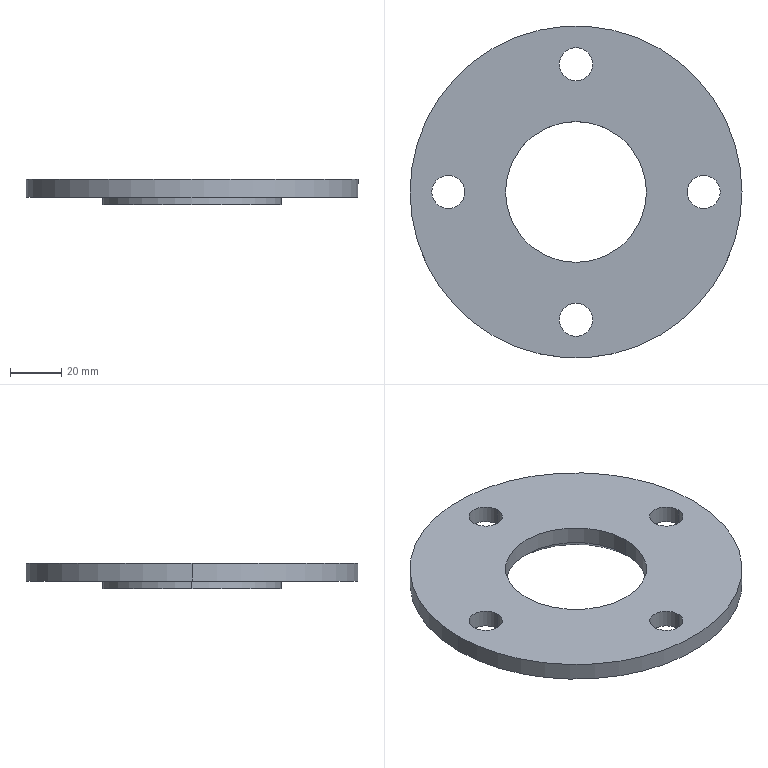Part | SolidWorks | features BaseBody 1 | 1 solid | 19 faces | box 130 x 130 x 10 mm | volume 76001 mm3 | cylinder 14 | plane 3 | cone 2 | commonest cylinder face diameters 13 x8 55.2 x2 70 x2 130 x2
STEP:
#1=CARTESIAN_POINT('',(27.6,0.,-7.));
#2=VERTEX_POINT('',#1);
#3=CARTESIAN_POINT('',(30.6,0.,-10.));
#4=VERTEX_POINT('',#3);
#5=CARTESIAN_POINT('',(30.6,0.,-10.));
#6=DIRECTION('',(0.7071,0.,-0.7071));
#7=VECTOR('',#6,1000.);
#8=LINE('',#5,#7);
#9=EDGE_CURVE('',#2,#4,#8,.T.);
#10=ORIENTED_EDGE('',*,*,#9,.F.);
#11=CARTESIAN_POINT('',(-27.6,0.,-7.));
#12=VERTEX_POINT('',#11);
#13=CARTESIAN_POINT('',(0.,0.,-7.));
#14=DIRECTION('',(0.,0.,-1.));
#15=DIRECTION('',(1.,0.,0.));
#16=AXIS2_PLACEMENT_3D('',#13,#14,#15);
#17=CIRCLE('',#16,27.6);
#18=EDGE_CURVE('',#12,#2,#17,.T.);
#19=ORIENTED_EDGE('',*,*,#18,.F.);
#20=CARTESIAN_POINT('',(-30.6,0.,-10.));
#21=VERTEX_POINT('',#20);
#22=CARTESIAN_POINT('',(-30.6,0.,-10.));
#23=DIRECTION('',(-0.7071,0.,-0.7071));
#24=VECTOR('',#23,1000.);
#25=LINE('',#22,#24);
#26=EDGE_CURVE('',#12,#21,#25,.T.);
#27=ORIENTED_EDGE('',*,*,#26,.T.);
#28=CARTESIAN_POINT('',(0.,0.,-10.));
#29=DIRECTION('',(0.,0.,1.));
#30=DIRECTION('',(1.,0.,0.));
#31=AXIS2_PLACEMENT_3D('',#28,#29,#30);
#32=CIRCLE('',#31,30.6);
#33=EDGE_CURVE('',#4,#21,#32,.T.);
#34=ORIENTED_EDGE('',*,*,#33,.F.);
#35=EDGE_LOOP('',(#10,#19,#27,#34));
#36=FACE_OUTER_BOUND('',#35,.T.);
#37=CARTESIAN_POINT('',(0.,0.,-10.));
#38=DIRECTION('',(0.,0.,-1.));
#39=DIRECTION('',(-1.,0.,0.));
#40=AXIS2_PLACEMENT_3D('',#37,#38,#39);
#41=CONICAL_SURFACE('',#40,30.6,0.7854);
#42=ADVANCED_FACE('',(#36),#41,.F.);
#43=CARTESIAN_POINT('',(35.,0.,-7.));
#44=VERTEX_POINT('',#43);
#45=CARTESIAN_POINT('',(35.,0.,-10.));
#46=VERTEX_POINT('',#45);
#47=CARTESIAN_POINT('',(35.,0.,-7.));
#48=DIRECTION('',(0.,0.,-1.));
#49=VECTOR('',#48,1000.);
#50=LINE('',#47,#49);
#51=EDGE_CURVE('',#44,#46,#50,.T.);
#52=ORIENTED_EDGE('',*,*,#51,.F.);
#53=CARTESIAN_POINT('',(-35.,0.,-7.));
#54=VERTEX_POINT('',#53);
#55=CARTESIAN_POINT('',(0.,0.,-7.));
#56=DIRECTION('',(0.,0.,-1.));
#57=DIRECTION('',(-1.,0.,0.));
#58=AXIS2_PLACEMENT_3D('',#55,#56,#57);
#59=CIRCLE('',#58,35.);
#60=EDGE_CURVE('',#44,#54,#59,.T.);
#61=ORIENTED_EDGE('',*,*,#60,.T.);
#62=CARTESIAN_POINT('',(-35.,0.,-10.));
#63=VERTEX_POINT('',#62);
#64=CARTESIAN_POINT('',(-35.,0.,-7.));
#65=DIRECTION('',(0.,0.,-1.));
#66=VECTOR('',#65,1000.);
#67=LINE('',#64,#66);
#68=EDGE_CURVE('',#54,#63,#67,.T.);
#69=ORIENTED_EDGE('',*,*,#68,.T.);
#70=CARTESIAN_POINT('',(0.,0.,-10.));
#71=DIRECTION('',(0.,0.,-1.));
#72=DIRECTION('',(-1.,0.,0.));
#73=AXIS2_PLACEMENT_3D('',#70,#71,#72);
#74=CIRCLE('',#73,35.);
#75=EDGE_CURVE('',#46,#63,#74,.T.);
#76=ORIENTED_EDGE('',*,*,#75,.F.);
#77=EDGE_LOOP('',(#52,#61,#69,#76));
#78=FACE_OUTER_BOUND('',#77,.T.);
#79=CARTESIAN_POINT('',(0.,0.,-7.));
#80=DIRECTION('',(0.,0.,-1.));
#81=DIRECTION('',(-1.,0.,0.));
#82=AXIS2_PLACEMENT_3D('',#79,#80,#81);
#83=CYLINDRICAL_SURFACE('',#82,35.);
#84=ADVANCED_FACE('',(#78),#83,.T.);
#85=CARTESIAN_POINT('',(6.5,50.,-7.));
#86=VERTEX_POINT('',#85);
#87=CARTESIAN_POINT('',(-6.5,50.,-7.));
#88=VERTEX_POINT('',#87);
#89=CARTESIAN_POINT('',(0.,50.,-7.));
#90=DIRECTION('',(0.,0.,1.));
#91=DIRECTION('',(-1.,0.,0.));
#92=AXIS2_PLACEMENT_3D('',#89,#90,#91);
#93=CIRCLE('',#92,6.5);
#94=EDGE_CURVE('',#86,#88,#93,.T.);
#95=ORIENTED_EDGE('',*,*,#94,.T.);
#96=CARTESIAN_POINT('',(0.,50.,-7.));
#97=DIRECTION('',(0.,0.,1.));
#98=DIRECTION('',(-1.,0.,0.));
#99=AXIS2_PLACEMENT_3D('',#96,#97,#98);
#100=CIRCLE('',#99,6.5);
#101=EDGE_CURVE('',#88,#86,#100,.T.);
#102=ORIENTED_EDGE('',*,*,#101,.T.);
#103=EDGE_LOOP('',(#95,#102));
#104=FACE_BOUND('',#103,.T.);
#105=CARTESIAN_POINT('',(56.5,0.,-7.));
#106=VERTEX_POINT('',#105);
#107=CARTESIAN_POINT('',(43.5,0.,-7.));
#108=VERTEX_POINT('',#107);
#109=CARTESIAN_POINT('',(50.,0.,-7.));
#110=DIRECTION('',(0.,0.,1.));
#111=DIRECTION('',(-1.,0.,0.));
#112=AXIS2_PLACEMENT_3D('',#109,#110,#111);
#113=CIRCLE('',#112,6.5);
#114=EDGE_CURVE('',#106,#108,#113,.T.);
#115=ORIENTED_EDGE('',*,*,#114,.T.);
#116=CARTESIAN_POINT('',(50.,0.,-7.));
#117=DIRECTION('',(0.,0.,1.));
#118=DIRECTION('',(-1.,0.,0.));
#119=AXIS2_PLACEMENT_3D('',#116,#117,#118);
#120=CIRCLE('',#119,6.5);
#121=EDGE_CURVE('',#108,#106,#120,.T.);
#122=ORIENTED_EDGE('',*,*,#121,.T.);
#123=EDGE_LOOP('',(#115,#122));
#124=FACE_BOUND('',#123,.T.);
#125=CARTESIAN_POINT('',(6.5,-50.,-7.));
#126=VERTEX_POINT('',#125);
#127=CARTESIAN_POINT('',(-6.5,-50.,-7.));
#128=VERTEX_POINT('',#127);
#129=CARTESIAN_POINT('',(0.,-50.,-7.));
#130=DIRECTION('',(0.,0.,1.));
#131=DIRECTION('',(-1.,0.,0.));
#132=AXIS2_PLACEMENT_3D('',#129,#130,#131);
#133=CIRCLE('',#132,6.5);
#134=EDGE_CURVE('',#126,#128,#133,.T.);
#135=ORIENTED_EDGE('',*,*,#134,.T.);
#136=CARTESIAN_POINT('',(0.,-50.,-7.));
#137=DIRECTION('',(0.,0.,1.));
#138=DIRECTION('',(-1.,0.,0.));
#139=AXIS2_PLACEMENT_3D('',#136,#137,#138);
#140=CIRCLE('',#139,6.5);
#141=EDGE_CURVE('',#128,#126,#140,.T.);
#142=ORIENTED_EDGE('',*,*,#141,.T.);
#143=EDGE_LOOP('',(#135,#142));
#144=FACE_BOUND('',#143,.T.);
#145=CARTESIAN_POINT('',(-43.5,0.,-7.));
#146=VERTEX_POINT('',#145);
#147=CARTESIAN_POINT('',(-56.5,0.,-7.));
#148=VERTEX_POINT('',#147);
#149=CARTESIAN_POINT('',(-50.,0.,-7.));
#150=DIRECTION('',(0.,0.,1.));
#151=DIRECTION('',(-1.,0.,0.));
#152=AXIS2_PLACEMENT_3D('',#149,#150,#151);
#153=CIRCLE('',#152,6.5);
#154=EDGE_CURVE('',#146,#148,#153,.T.);
#155=ORIENTED_EDGE('',*,*,#154,.T.);
#156=CARTESIAN_POINT('',(-50.,0.,-7.));
#157=DIRECTION('',(0.,0.,1.));
#158=DIRECTION('',(-1.,0.,0.));
#159=AXIS2_PLACEMENT_3D('',#156,#157,#158);
#160=CIRCLE('',#159,6.5);
#161=EDGE_CURVE('',#148,#146,#160,.T.);
#162=ORIENTED_EDGE('',*,*,#161,.T.);
#163=EDGE_LOOP('',(#155,#162));
#164=FACE_BOUND('',#163,.T.);
#165=CARTESIAN_POINT('',(0.,0.,-7.));
#166=DIRECTION('',(0.,0.,-1.));
#167=DIRECTION('',(-1.,0.,0.));
#168=AXIS2_PLACEMENT_3D('',#165,#166,#167);
#169=CIRCLE('',#168,35.);
#170=EDGE_CURVE('',#54,#44,#169,.T.);
#171=ORIENTED_EDGE('',*,*,#170,.F.);
#172=ORIENTED_EDGE('',*,*,#60,.F.);
#173=EDGE_LOOP('',(#171,#172));
#174=FACE_BOUND('',#173,.T.);
#175=CARTESIAN_POINT('',(65.,0.,-7.));
#176=VERTEX_POINT('',#175);
#177=CARTESIAN_POINT('',(-65.,0.,-7.));
#178=VERTEX_POINT('',#177);
#179=CARTESIAN_POINT('',(0.,0.,-7.));
#180=DIRECTION('',(0.,0.,-1.));
#181=DIRECTION('',(-1.,0.,0.));
#182=AXIS2_PLACEMENT_3D('',#179,#180,#181);
#183=CIRCLE('',#182,65.);
#184=EDGE_CURVE('',#176,#178,#183,.T.);
#185=ORIENTED_EDGE('',*,*,#184,.T.);
#186=CARTESIAN_POINT('',(0.,0.,-7.));
#187=DIRECTION('',(0.,0.,-1.));
#188=DIRECTION('',(-1.,0.,0.));
#189=AXIS2_PLACEMENT_3D('',#186,#187,#188);
#190=CIRCLE('',#189,65.);
#191=EDGE_CURVE('',#178,#176,#190,.T.);
#192=ORIENTED_EDGE('',*,*,#191,.T.);
#193=EDGE_LOOP('',(#185,#192));
#194=FACE_OUTER_BOUND('',#193,.T.);
#195=CARTESIAN_POINT('',(0.,0.,-7.));
#196=DIRECTION('',(0.,0.,-1.));
#197=DIRECTION('',(0.,-1.,0.));
#198=AXIS2_PLACEMENT_3D('',#195,#196,#197);
#199=PLANE('',#198);
#200=ADVANCED_FACE('',(#104,#124,#144,#164,#174,#194),#199,.T.);
#201=CARTESIAN_POINT('',(-27.6,0.,0.));
#202=VERTEX_POINT('',#201);
#203=CARTESIAN_POINT('',(-27.6,0.,-10.));
#204=DIRECTION('',(0.,0.,1.));
#205=VECTOR('',#204,1000.);
#206=LINE('',#203,#205);
#207=EDGE_CURVE('',#12,#202,#206,.T.);
#208=ORIENTED_EDGE('',*,*,#207,.F.);
#209=ORIENTED_EDGE('',*,*,#18,.T.);
#210=CARTESIAN_POINT('',(27.6,0.,0.));
#211=VERTEX_POINT('',#210);
#212=CARTESIAN_POINT('',(27.6,0.,-10.));
#213=DIRECTION('',(0.,0.,1.));
#214=VECTOR('',#213,1000.);
#215=LINE('',#212,#214);
#216=EDGE_CURVE('',#2,#211,#215,.T.);
#217=ORIENTED_EDGE('',*,*,#216,.T.);
#218=CARTESIAN_POINT('',(0.,0.,0.));
#219=DIRECTION('',(0.,0.,1.));
#220=DIRECTION('',(1.,0.,0.));
#221=AXIS2_PLACEMENT_3D('',#218,#219,#220);
#222=CIRCLE('',#221,27.6);
#223=EDGE_CURVE('',#211,#202,#222,.T.);
#224=ORIENTED_EDGE('',*,*,#223,.T.);
#225=EDGE_LOOP('',(#208,#209,#217,#224));
#226=FACE_OUTER_BOUND('',#225,.T.);
#227=CARTESIAN_POINT('',(0.,0.,-10.));
#228=DIRECTION('',(0.,0.,1.));
#229=DIRECTION('',(1.,0.,0.));
#230=AXIS2_PLACEMENT_3D('',#227,#228,#229);
#231=CYLINDRICAL_SURFACE('',#230,27.6);
#232=ADVANCED_FACE('',(#226),#231,.F.);
#233=ORIENTED_EDGE('',*,*,#223,.F.);
#234=CARTESIAN_POINT('',(0.,0.,0.));
#235=DIRECTION('',(0.,0.,1.));
#236=DIRECTION('',(1.,0.,0.));
#237=AXIS2_PLACEMENT_3D('',#234,#235,#236);
#238=CIRCLE('',#237,27.6);
#239=EDGE_CURVE('',#202,#211,#238,.T.);
#240=ORIENTED_EDGE('',*,*,#239,.F.);
#241=EDGE_LOOP('',(#233,#240));
#242=FACE_BOUND('',#241,.T.);
#243=CARTESIAN_POINT('',(6.5,50.,0.));
#244=VERTEX_POINT('',#243);
#245=CARTESIAN_POINT('',(-6.5,50.,0.));
#246=VERTEX_POINT('',#245);
#247=CARTESIAN_POINT('',(0.,50.,0.));
#248=DIRECTION('',(0.,0.,1.));
#249=DIRECTION('',(1.,0.,0.));
#250=AXIS2_PLACEMENT_3D('',#247,#248,#249);
#251=CIRCLE('',#250,6.5);
#252=EDGE_CURVE('',#244,#246,#251,.T.);
#253=ORIENTED_EDGE('',*,*,#252,.F.);
#254=CARTESIAN_POINT('',(0.,50.,0.));
#255=DIRECTION('',(0.,0.,1.));
#256=DIRECTION('',(1.,0.,0.));
#257=AXIS2_PLACEMENT_3D('',#254,#255,#256);
#258=CIRCLE('',#257,6.5);
#259=EDGE_CURVE('',#246,#244,#258,.T.);
#260=ORIENTED_EDGE('',*,*,#259,.F.);
#261=EDGE_LOOP('',(#253,#260));
#262=FACE_BOUND('',#261,.T.);
#263=CARTESIAN_POINT('',(56.5,0.,0.));
#264=VERTEX_POINT('',#263);
#265=CARTESIAN_POINT('',(43.5,0.,0.));
#266=VERTEX_POINT('',#265);
#267=CARTESIAN_POINT('',(50.,0.,0.));
#268=DIRECTION('',(0.,0.,1.));
#269=DIRECTION('',(0.,-1.,0.));
#270=AXIS2_PLACEMENT_3D('',#267,#268,#269);
#271=CIRCLE('',#270,6.5);
#272=EDGE_CURVE('',#264,#266,#271,.T.);
#273=ORIENTED_EDGE('',*,*,#272,.F.);
#274=CARTESIAN_POINT('',(50.,0.,0.));
#275=DIRECTION('',(0.,0.,1.));
#276=DIRECTION('',(0.,-1.,0.));
#277=AXIS2_PLACEMENT_3D('',#274,#275,#276);
#278=CIRCLE('',#277,6.5);
#279=EDGE_CURVE('',#266,#264,#278,.T.);
#280=ORIENTED_EDGE('',*,*,#279,.F.);
#281=EDGE_LOOP('',(#273,#280));
#282=FACE_BOUND('',#281,.T.);
#283=CARTESIAN_POINT('',(6.5,-50.,0.));
#284=VERTEX_POINT('',#283);
#285=CARTESIAN_POINT('',(-6.5,-50.,0.));
#286=VERTEX_POINT('',#285);
#287=CARTESIAN_POINT('',(0.,-50.,0.));
#288=DIRECTION('',(0.,0.,1.));
#289=DIRECTION('',(-1.,0.,0.));
#290=AXIS2_PLACEMENT_3D('',#287,#288,#289);
#291=CIRCLE('',#290,6.5);
#292=EDGE_CURVE('',#284,#286,#291,.T.);
#293=ORIENTED_EDGE('',*,*,#292,.F.);
#294=CARTESIAN_POINT('',(0.,-50.,0.));
#295=DIRECTION('',(0.,0.,1.));
#296=DIRECTION('',(-1.,0.,0.));
#297=AXIS2_PLACEMENT_3D('',#294,#295,#296);
#298=CIRCLE('',#297,6.5);
#299=EDGE_CURVE('',#286,#284,#298,.T.);
#300=ORIENTED_EDGE('',*,*,#299,.F.);
#301=EDGE_LOOP('',(#293,#300));
#302=FACE_BOUND('',#301,.T.);
#303=CARTESIAN_POINT('',(-43.5,0.,0.));
#304=VERTEX_POINT('',#303);
#305=CARTESIAN_POINT('',(-56.5,0.,0.));
#306=VERTEX_POINT('',#305);
#307=CARTESIAN_POINT('',(-50.,0.,0.));
#308=DIRECTION('',(0.,0.,1.));
#309=DIRECTION('',(0.,1.,0.));
#310=AXIS2_PLACEMENT_3D('',#307,#308,#309);
#311=CIRCLE('',#310,6.5);
#312=EDGE_CURVE('',#304,#306,#311,.T.);
#313=ORIENTED_EDGE('',*,*,#312,.F.);
#314=CARTESIAN_POINT('',(-50.,0.,0.));
#315=DIRECTION('',(0.,0.,1.));
#316=DIRECTION('',(0.,1.,0.));
#317=AXIS2_PLACEMENT_3D('',#314,#315,#316);
#318=CIRCLE('',#317,6.5);
#319=EDGE_CURVE('',#306,#304,#318,.T.);
#320=ORIENTED_EDGE('',*,*,#319,.F.);
#321=EDGE_LOOP('',(#313,#320));
#322=FACE_BOUND('',#321,.T.);
#323=CARTESIAN_POINT('',(65.,0.,0.));
#324=VERTEX_POINT('',#323);
#325=CARTESIAN_POINT('',(-65.,0.,0.));
#326=VERTEX_POINT('',#325);
#327=CARTESIAN_POINT('',(0.,0.,0.));
#328=DIRECTION('',(0.,0.,1.));
#329=DIRECTION('',(1.,0.,0.));
#330=AXIS2_PLACEMENT_3D('',#327,#328,#329);
#331=CIRCLE('',#330,65.);
#332=EDGE_CURVE('',#324,#326,#331,.T.);
#333=ORIENTED_EDGE('',*,*,#332,.T.);
#334=CARTESIAN_POINT('',(0.,0.,0.));
#335=DIRECTION('',(0.,0.,1.));
#336=DIRECTION('',(1.,0.,0.));
#337=AXIS2_PLACEMENT_3D('',#334,#335,#336);
#338=CIRCLE('',#337,65.);
#339=EDGE_CURVE('',#326,#324,#338,.T.);
#340=ORIENTED_EDGE('',*,*,#339,.T.);
#341=EDGE_LOOP('',(#333,#340));
#342=FACE_OUTER_BOUND('',#341,.T.);
#343=CARTESIAN_POINT('',(0.,0.,0.));
#344=DIRECTION('',(0.,0.,1.));
#345=DIRECTION('',(1.,0.,0.));
#346=AXIS2_PLACEMENT_3D('',#343,#344,#345);
#347=PLANE('',#346);
#348=ADVANCED_FACE('',(#242,#262,#282,#302,#322,#342),#347,.T.);
#349=CARTESIAN_POINT('',(-56.5,0.,-10.));
#350=DIRECTION('',(0.,0.,1.));
#351=VECTOR('',#350,1000.);
#352=LINE('',#349,#351);
#353=EDGE_CURVE('',#148,#306,#352,.T.);
#354=ORIENTED_EDGE('',*,*,#353,.F.);
#355=ORIENTED_EDGE('',*,*,#154,.F.);
#356=CARTESIAN_POINT('',(-43.5,0.,-10.));
#357=DIRECTION('',(0.,0.,1.));
#358=VECTOR('',#357,1000.);
#359=LINE('',#356,#358);
#360=EDGE_CURVE('',#146,#304,#359,.T.);
#361=ORIENTED_EDGE('',*,*,#360,.T.);
#362=ORIENTED_EDGE('',*,*,#312,.T.);
#363=EDGE_LOOP('',(#354,#355,#361,#362));
#364=FACE_OUTER_BOUND('',#363,.T.);
#365=CARTESIAN_POINT('',(-50.,0.,-10.));
#366=DIRECTION('',(0.,0.,1.));
#367=DIRECTION('',(1.,0.,0.));
#368=AXIS2_PLACEMENT_3D('',#365,#366,#367);
#369=CYLINDRICAL_SURFACE('',#368,6.5);
#370=ADVANCED_FACE('',(#364),#369,.F.);
#371=CARTESIAN_POINT('',(-6.5,-50.,-10.));
#372=DIRECTION('',(0.,0.,1.));
#373=VECTOR('',#372,1000.);
#374=LINE('',#371,#373);
#375=EDGE_CURVE('',#128,#286,#374,.T.);
#376=ORIENTED_EDGE('',*,*,#375,.F.);
#377=ORIENTED_EDGE('',*,*,#134,.F.);
#378=CARTESIAN_POINT('',(6.5,-50.,-10.));
#379=DIRECTION('',(0.,0.,1.));
#380=VECTOR('',#379,1000.);
#381=LINE('',#378,#380);
#382=EDGE_CURVE('',#126,#284,#381,.T.);
#383=ORIENTED_EDGE('',*,*,#382,.T.);
#384=ORIENTED_EDGE('',*,*,#292,.T.);
#385=EDGE_LOOP('',(#376,#377,#383,#384));
#386=FACE_OUTER_BOUND('',#385,.T.);
#387=CARTESIAN_POINT('',(0.,-50.,-10.));
#388=DIRECTION('',(0.,0.,1.));
#389=DIRECTION('',(1.,0.,0.));
#390=AXIS2_PLACEMENT_3D('',#387,#388,#389);
#391=CYLINDRICAL_SURFACE('',#390,6.5);
#392=ADVANCED_FACE('',(#386),#391,.F.);
#393=CARTESIAN_POINT('',(43.5,0.,-10.));
#394=DIRECTION('',(0.,0.,1.));
#395=VECTOR('',#394,1000.);
#396=LINE('',#393,#395);
#397=EDGE_CURVE('',#108,#266,#396,.T.);
#398=ORIENTED_EDGE('',*,*,#397,.F.);
#399=ORIENTED_EDGE('',*,*,#114,.F.);
#400=CARTESIAN_POINT('',(56.5,0.,-10.));
#401=DIRECTION('',(0.,0.,1.));
#402=VECTOR('',#401,1000.);
#403=LINE('',#400,#402);
#404=EDGE_CURVE('',#106,#264,#403,.T.);
#405=ORIENTED_EDGE('',*,*,#404,.T.);
#406=ORIENTED_EDGE('',*,*,#272,.T.);
#407=EDGE_LOOP('',(#398,#399,#405,#406));
#408=FACE_OUTER_BOUND('',#407,.T.);
#409=CARTESIAN_POINT('',(50.,0.,-10.));
#410=DIRECTION('',(0.,0.,1.));
#411=DIRECTION('',(1.,0.,0.));
#412=AXIS2_PLACEMENT_3D('',#409,#410,#411);
#413=CYLINDRICAL_SURFACE('',#412,6.5);
#414=ADVANCED_FACE('',(#408),#413,.F.);
#415=CARTESIAN_POINT('',(-6.5,50.,-10.));
#416=DIRECTION('',(0.,0.,1.));
#417=VECTOR('',#416,1000.);
#418=LINE('',#415,#417);
#419=EDGE_CURVE('',#88,#246,#418,.T.);
#420=ORIENTED_EDGE('',*,*,#419,.F.);
#421=ORIENTED_EDGE('',*,*,#94,.F.);
#422=CARTESIAN_POINT('',(6.5,50.,-10.));
#423=DIRECTION('',(0.,0.,1.));
#424=VECTOR('',#423,1000.);
#425=LINE('',#422,#424);
#426=EDGE_CURVE('',#86,#244,#425,.T.);
#427=ORIENTED_EDGE('',*,*,#426,.T.);
#428=ORIENTED_EDGE('',*,*,#252,.T.);
#429=EDGE_LOOP('',(#420,#421,#427,#428));
#430=FACE_OUTER_BOUND('',#429,.T.);
#431=CARTESIAN_POINT('',(0.,50.,-10.));
#432=DIRECTION('',(0.,0.,1.));
#433=DIRECTION('',(1.,0.,0.));
#434=AXIS2_PLACEMENT_3D('',#431,#432,#433);
#435=CYLINDRICAL_SURFACE('',#434,6.5);
#436=ADVANCED_FACE('',(#430),#435,.F.);
#437=CARTESIAN_POINT('',(0.,0.,-10.));
#438=DIRECTION('',(0.,0.,1.));
#439=DIRECTION('',(1.,0.,0.));
#440=AXIS2_PLACEMENT_3D('',#437,#438,#439);
#441=CIRCLE('',#440,30.6);
#442=EDGE_CURVE('',#21,#4,#441,.T.);
#443=ORIENTED_EDGE('',*,*,#442,.T.);
#444=ORIENTED_EDGE('',*,*,#33,.T.);
#445=EDGE_LOOP('',(#443,#444));
#446=FACE_BOUND('',#445,.T.);
#447=CARTESIAN_POINT('',(0.,0.,-10.));
#448=DIRECTION('',(0.,0.,-1.));
#449=DIRECTION('',(-1.,0.,0.));
#450=AXIS2_PLACEMENT_3D('',#447,#448,#449);
#451=CIRCLE('',#450,35.);
#452=EDGE_CURVE('',#63,#46,#451,.T.);
#453=ORIENTED_EDGE('',*,*,#452,.T.);
#454=ORIENTED_EDGE('',*,*,#75,.T.);
#455=EDGE_LOOP('',(#453,#454));
#456=FACE_OUTER_BOUND('',#455,.T.);
#457=CARTESIAN_POINT('',(0.,0.,-10.));
#458=DIRECTION('',(0.,0.,1.));
#459=DIRECTION('',(1.,0.,0.));
#460=AXIS2_PLACEMENT_3D('',#457,#458,#459);
#461=PLANE('',#460);
#462=ADVANCED_FACE('',(#446,#456),#461,.F.);
#463=CARTESIAN_POINT('',(-65.,0.,-10.));
#464=DIRECTION('',(0.,0.,1.));
#465=VECTOR('',#464,1000.);
#466=LINE('',#463,#465);
#467=EDGE_CURVE('',#178,#326,#466,.T.);
#468=ORIENTED_EDGE('',*,*,#467,.F.);
#469=ORIENTED_EDGE('',*,*,#184,.F.);
#470=CARTESIAN_POINT('',(65.,0.,-10.));
#471=DIRECTION('',(0.,0.,1.));
#472=VECTOR('',#471,1000.);
#473=LINE('',#470,#472);
#474=EDGE_CURVE('',#176,#324,#473,.T.);
#475=ORIENTED_EDGE('',*,*,#474,.T.);
#476=ORIENTED_EDGE('',*,*,#339,.F.);
#477=EDGE_LOOP('',(#468,#469,#475,#476));
#478=FACE_OUTER_BOUND('',#477,.T.);
#479=CARTESIAN_POINT('',(0.,0.,-10.));
#480=DIRECTION('',(0.,0.,1.));
#481=DIRECTION('',(1.,0.,0.));
#482=AXIS2_PLACEMENT_3D('',#479,#480,#481);
#483=CYLINDRICAL_SURFACE('',#482,65.);
#484=ADVANCED_FACE('',(#478),#483,.T.);
#485=ORIENTED_EDGE('',*,*,#191,.F.);
#486=ORIENTED_EDGE('',*,*,#467,.T.);
#487=ORIENTED_EDGE('',*,*,#332,.F.);
#488=ORIENTED_EDGE('',*,*,#474,.F.);
#489=EDGE_LOOP('',(#485,#486,#487,#488));
#490=FACE_OUTER_BOUND('',#489,.T.);
#491=CARTESIAN_POINT('',(0.,0.,-10.));
#492=DIRECTION('',(0.,0.,1.));
#493=DIRECTION('',(1.,0.,0.));
#494=AXIS2_PLACEMENT_3D('',#491,#492,#493);
#495=CYLINDRICAL_SURFACE('',#494,65.);
#496=ADVANCED_FACE('',(#490),#495,.T.);
#497=ORIENTED_EDGE('',*,*,#101,.F.);
#498=ORIENTED_EDGE('',*,*,#419,.T.);
#499=ORIENTED_EDGE('',*,*,#259,.T.);
#500=ORIENTED_EDGE('',*,*,#426,.F.);
#501=EDGE_LOOP('',(#497,#498,#499,#500));
#502=FACE_OUTER_BOUND('',#501,.T.);
#503=CARTESIAN_POINT('',(0.,50.,-10.));
#504=DIRECTION('',(0.,0.,1.));
#505=DIRECTION('',(1.,0.,0.));
#506=AXIS2_PLACEMENT_3D('',#503,#504,#505);
#507=CYLINDRICAL_SURFACE('',#506,6.5);
#508=ADVANCED_FACE('',(#502),#507,.F.);
#509=ORIENTED_EDGE('',*,*,#121,.F.);
#510=ORIENTED_EDGE('',*,*,#397,.T.);
#511=ORIENTED_EDGE('',*,*,#279,.T.);
#512=ORIENTED_EDGE('',*,*,#404,.F.);
#513=EDGE_LOOP('',(#509,#510,#511,#512));
#514=FACE_OUTER_BOUND('',#513,.T.);
#515=CARTESIAN_POINT('',(50.,0.,-10.));
#516=DIRECTION('',(0.,0.,1.));
#517=DIRECTION('',(1.,0.,0.));
#518=AXIS2_PLACEMENT_3D('',#515,#516,#517);
#519=CYLINDRICAL_SURFACE('',#518,6.5);
#520=ADVANCED_FACE('',(#514),#519,.F.);
#521=ORIENTED_EDGE('',*,*,#141,.F.);
#522=ORIENTED_EDGE('',*,*,#375,.T.);
#523=ORIENTED_EDGE('',*,*,#299,.T.);
#524=ORIENTED_EDGE('',*,*,#382,.F.);
#525=EDGE_LOOP('',(#521,#522,#523,#524));
#526=FACE_OUTER_BOUND('',#525,.T.);
#527=CARTESIAN_POINT('',(0.,-50.,-10.));
#528=DIRECTION('',(0.,0.,1.));
#529=DIRECTION('',(1.,0.,0.));
#530=AXIS2_PLACEMENT_3D('',#527,#528,#529);
#531=CYLINDRICAL_SURFACE('',#530,6.5);
#532=ADVANCED_FACE('',(#526),#531,.F.);
#533=ORIENTED_EDGE('',*,*,#161,.F.);
#534=ORIENTED_EDGE('',*,*,#353,.T.);
#535=ORIENTED_EDGE('',*,*,#319,.T.);
#536=ORIENTED_EDGE('',*,*,#360,.F.);
#537=EDGE_LOOP('',(#533,#534,#535,#536));
#538=FACE_OUTER_BOUND('',#537,.T.);
#539=CARTESIAN_POINT('',(-50.,0.,-10.));
#540=DIRECTION('',(0.,0.,1.));
#541=DIRECTION('',(1.,0.,0.));
#542=AXIS2_PLACEMENT_3D('',#539,#540,#541);
#543=CYLINDRICAL_SURFACE('',#542,6.5);
#544=ADVANCED_FACE('',(#538),#543,.F.);
#545=CARTESIAN_POINT('',(0.,0.,-7.));
#546=DIRECTION('',(0.,0.,-1.));
#547=DIRECTION('',(1.,0.,0.));
#548=AXIS2_PLACEMENT_3D('',#545,#546,#547);
#549=CIRCLE('',#548,27.6);
#550=EDGE_CURVE('',#2,#12,#549,.T.);
#551=ORIENTED_EDGE('',*,*,#550,.T.);
#552=ORIENTED_EDGE('',*,*,#207,.T.);
#553=ORIENTED_EDGE('',*,*,#239,.T.);
#554=ORIENTED_EDGE('',*,*,#216,.F.);
#555=EDGE_LOOP('',(#551,#552,#553,#554));
#556=FACE_OUTER_BOUND('',#555,.T.);
#557=CARTESIAN_POINT('',(0.,0.,-10.));
#558=DIRECTION('',(0.,0.,1.));
#559=DIRECTION('',(1.,0.,0.));
#560=AXIS2_PLACEMENT_3D('',#557,#558,#559);
#561=CYLINDRICAL_SURFACE('',#560,27.6);
#562=ADVANCED_FACE('',(#556),#561,.F.);
#563=ORIENTED_EDGE('',*,*,#170,.T.);
#564=ORIENTED_EDGE('',*,*,#51,.T.);
#565=ORIENTED_EDGE('',*,*,#452,.F.);
#566=ORIENTED_EDGE('',*,*,#68,.F.);
#567=EDGE_LOOP('',(#563,#564,#565,#566));
#568=FACE_OUTER_BOUND('',#567,.T.);
#569=CARTESIAN_POINT('',(0.,0.,-7.));
#570=DIRECTION('',(0.,0.,-1.));
#571=DIRECTION('',(-1.,0.,0.));
#572=AXIS2_PLACEMENT_3D('',#569,#570,#571);
#573=CYLINDRICAL_SURFACE('',#572,35.);
#574=ADVANCED_FACE('',(#568),#573,.T.);
#575=ORIENTED_EDGE('',*,*,#550,.F.);
#576=ORIENTED_EDGE('',*,*,#9,.T.);
#577=ORIENTED_EDGE('',*,*,#442,.F.);
#578=ORIENTED_EDGE('',*,*,#26,.F.);
#579=EDGE_LOOP('',(#575,#576,#577,#578));
#580=FACE_OUTER_BOUND('',#579,.T.);
#581=CARTESIAN_POINT('',(0.,0.,-10.));
#582=DIRECTION('',(0.,0.,-1.));
#583=DIRECTION('',(-1.,0.,0.));
#584=AXIS2_PLACEMENT_3D('',#581,#582,#583);
#585=CONICAL_SURFACE('',#584,30.6,0.7854);
#586=ADVANCED_FACE('',(#580),#585,.F.);
#587=CLOSED_SHELL('',(#42,#84,#200,#232,#348,#370,#392,#414,#436,#462,#484,#496,#508,#520,#532,#544,#562,#574,#586));
#588=MANIFOLD_SOLID_BREP('',#587);
#589=CARTESIAN_POINT('',(0.,0.,0.));
#590=DIRECTION('',(0.,0.,1.));
#591=DIRECTION('',(1.,0.,0.));
#592=AXIS2_PLACEMENT_3D('',#589,#590,#591);
#593=(LENGTH_UNIT()NAMED_UNIT(*)SI_UNIT(.MILLI.,.METRE.));
#594=UNCERTAINTY_MEASURE_WITH_UNIT(LENGTH_MEASURE(0.00001),#593,'','');
#595=(NAMED_UNIT(*)PLANE_ANGLE_UNIT()SI_UNIT($,.RADIAN.));
#596=(NAMED_UNIT(*)SI_UNIT($,.STERADIAN.)SOLID_ANGLE_UNIT());
#597=(GEOMETRIC_REPRESENTATION_CONTEXT(3)GLOBAL_UNCERTAINTY_ASSIGNED_CONTEXT((#594))GLOBAL_UNIT_ASSIGNED_CONTEXT((#593,#595,#596))REPRESENTATION_CONTEXT('',''));
#598=ADVANCED_BREP_SHAPE_REPRESENTATION('',(#588,#592),#597);